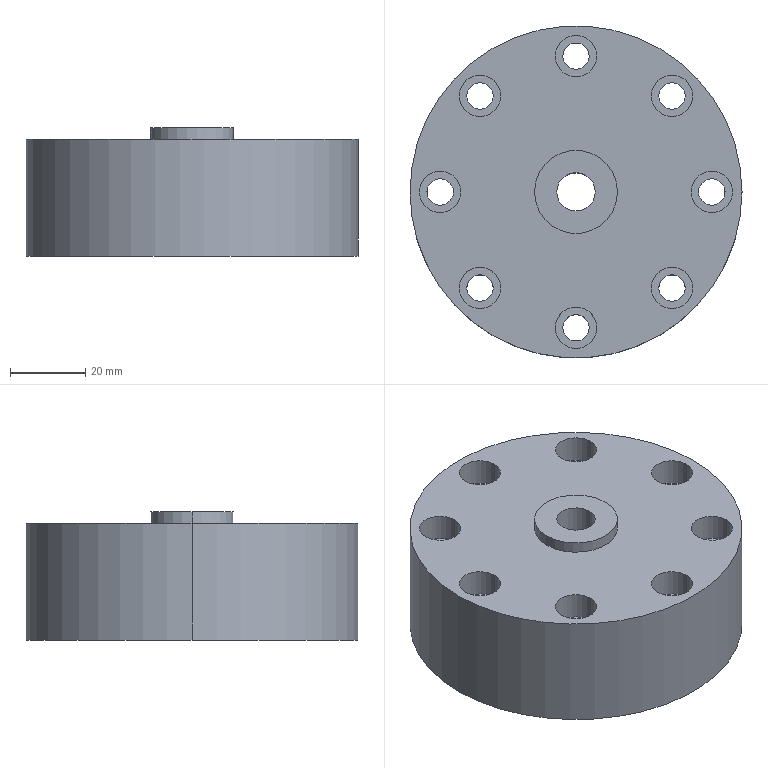Part | SolidWorks | features BaseBody 1 | 1 solid | 49 faces | box 88 x 88 x 34 mm | volume 174107 mm3 | cylinder 38 | plane 11 | commonest cylinder face diameters 7 x16 11 x16 10.2 x2 22 x2 88 x2
STEP:
#1=CARTESIAN_POINT('',(-44.,-15.,364.481));
#2=VERTEX_POINT('',#1);
#3=CARTESIAN_POINT('',(44.,-15.,364.481));
#4=VERTEX_POINT('',#3);
#5=CARTESIAN_POINT('',(0.,-15.,364.481));
#6=DIRECTION('',(0.,0.,-1.));
#7=DIRECTION('',(-1.,0.,0.));
#8=AXIS2_PLACEMENT_3D('',#5,#6,#7);
#9=CIRCLE('',#8,44.);
#10=EDGE_CURVE('',#2,#4,#9,.T.);
#11=ORIENTED_EDGE('',*,*,#10,.T.);
#12=CARTESIAN_POINT('',(44.,-15.,333.481));
#13=VERTEX_POINT('',#12);
#14=CARTESIAN_POINT('',(44.,-15.,364.481));
#15=DIRECTION('',(0.,0.,-1.));
#16=VECTOR('',#15,1000.);
#17=LINE('',#14,#16);
#18=EDGE_CURVE('',#4,#13,#17,.T.);
#19=ORIENTED_EDGE('',*,*,#18,.T.);
#20=CARTESIAN_POINT('',(-44.,-15.,333.481));
#21=VERTEX_POINT('',#20);
#22=CARTESIAN_POINT('',(0.,-15.,333.481));
#23=DIRECTION('',(0.,0.,1.));
#24=DIRECTION('',(-1.,0.,0.));
#25=AXIS2_PLACEMENT_3D('',#22,#23,#24);
#26=CIRCLE('',#25,44.);
#27=EDGE_CURVE('',#13,#21,#26,.T.);
#28=ORIENTED_EDGE('',*,*,#27,.T.);
#29=CARTESIAN_POINT('',(-44.,-15.,364.481));
#30=DIRECTION('',(0.,0.,-1.));
#31=VECTOR('',#30,1000.);
#32=LINE('',#29,#31);
#33=EDGE_CURVE('',#2,#21,#32,.T.);
#34=ORIENTED_EDGE('',*,*,#33,.F.);
#35=EDGE_LOOP('',(#11,#19,#28,#34));
#36=FACE_OUTER_BOUND('',#35,.T.);
#37=CARTESIAN_POINT('',(0.,-15.,364.481));
#38=DIRECTION('',(0.,0.,-1.));
#39=DIRECTION('',(-1.,0.,0.));
#40=AXIS2_PLACEMENT_3D('',#37,#38,#39);
#41=CYLINDRICAL_SURFACE('',#40,44.);
#42=ADVANCED_FACE('',(#36),#41,.T.);
#43=CARTESIAN_POINT('',(5.1,-15.,333.481));
#44=VERTEX_POINT('',#43);
#45=CARTESIAN_POINT('',(-5.1,-15.,333.481));
#46=VERTEX_POINT('',#45);
#47=CARTESIAN_POINT('',(0.,-15.,333.481));
#48=DIRECTION('',(0.,0.,-1.));
#49=DIRECTION('',(1.,0.,0.));
#50=AXIS2_PLACEMENT_3D('',#47,#48,#49);
#51=CIRCLE('',#50,5.1);
#52=EDGE_CURVE('',#44,#46,#51,.T.);
#53=ORIENTED_EDGE('',*,*,#52,.T.);
#54=CARTESIAN_POINT('',(-5.1,-15.,367.481));
#55=VERTEX_POINT('',#54);
#56=CARTESIAN_POINT('',(-5.1,-15.,367.481));
#57=DIRECTION('',(0.,0.,1.));
#58=VECTOR('',#57,1000.);
#59=LINE('',#56,#58);
#60=EDGE_CURVE('',#46,#55,#59,.T.);
#61=ORIENTED_EDGE('',*,*,#60,.T.);
#62=CARTESIAN_POINT('',(5.1,-15.,367.481));
#63=VERTEX_POINT('',#62);
#64=CARTESIAN_POINT('',(0.,-15.,367.481));
#65=DIRECTION('',(0.,0.,-1.));
#66=DIRECTION('',(1.,0.,0.));
#67=AXIS2_PLACEMENT_3D('',#64,#65,#66);
#68=CIRCLE('',#67,5.1);
#69=EDGE_CURVE('',#63,#55,#68,.T.);
#70=ORIENTED_EDGE('',*,*,#69,.F.);
#71=CARTESIAN_POINT('',(5.1,-15.,367.481));
#72=DIRECTION('',(0.,0.,1.));
#73=VECTOR('',#72,1000.);
#74=LINE('',#71,#73);
#75=EDGE_CURVE('',#44,#63,#74,.T.);
#76=ORIENTED_EDGE('',*,*,#75,.F.);
#77=EDGE_LOOP('',(#53,#61,#70,#76));
#78=FACE_OUTER_BOUND('',#77,.T.);
#79=CARTESIAN_POINT('',(0.,-15.,367.481));
#80=DIRECTION('',(0.,0.,1.));
#81=DIRECTION('',(1.,0.,0.));
#82=AXIS2_PLACEMENT_3D('',#79,#80,#81);
#83=CYLINDRICAL_SURFACE('',#82,5.1);
#84=ADVANCED_FACE('',(#78),#83,.F.);
#85=CARTESIAN_POINT('',(39.5,-15.,333.481));
#86=VERTEX_POINT('',#85);
#87=CARTESIAN_POINT('',(32.5,-15.,333.481));
#88=VERTEX_POINT('',#87);
#89=CARTESIAN_POINT('',(36.,-15.,333.481));
#90=DIRECTION('',(0.,0.,-1.));
#91=DIRECTION('',(1.,0.,0.));
#92=AXIS2_PLACEMENT_3D('',#89,#90,#91);
#93=CIRCLE('',#92,3.5);
#94=EDGE_CURVE('',#86,#88,#93,.T.);
#95=ORIENTED_EDGE('',*,*,#94,.T.);
#96=CARTESIAN_POINT('',(32.5,-15.,357.281));
#97=VERTEX_POINT('',#96);
#98=CARTESIAN_POINT('',(32.5,-15.,333.481));
#99=DIRECTION('',(0.,0.,1.));
#100=VECTOR('',#99,1000.);
#101=LINE('',#98,#100);
#102=EDGE_CURVE('',#88,#97,#101,.T.);
#103=ORIENTED_EDGE('',*,*,#102,.T.);
#104=CARTESIAN_POINT('',(39.5,-15.,357.281));
#105=VERTEX_POINT('',#104);
#106=CARTESIAN_POINT('',(36.,-15.,357.281));
#107=DIRECTION('',(0.,0.,-1.));
#108=DIRECTION('',(1.,0.,0.));
#109=AXIS2_PLACEMENT_3D('',#106,#107,#108);
#110=CIRCLE('',#109,3.5);
#111=EDGE_CURVE('',#105,#97,#110,.T.);
#112=ORIENTED_EDGE('',*,*,#111,.F.);
#113=CARTESIAN_POINT('',(39.5,-15.,333.481));
#114=DIRECTION('',(0.,0.,1.));
#115=VECTOR('',#114,1000.);
#116=LINE('',#113,#115);
#117=EDGE_CURVE('',#86,#105,#116,.T.);
#118=ORIENTED_EDGE('',*,*,#117,.F.);
#119=EDGE_LOOP('',(#95,#103,#112,#118));
#120=FACE_OUTER_BOUND('',#119,.T.);
#121=CARTESIAN_POINT('',(36.,-15.,333.481));
#122=DIRECTION('',(0.,0.,1.));
#123=DIRECTION('',(1.,0.,0.));
#124=AXIS2_PLACEMENT_3D('',#121,#122,#123);
#125=CYLINDRICAL_SURFACE('',#124,3.5);
#126=ADVANCED_FACE('',(#120),#125,.F.);
#127=CARTESIAN_POINT('',(28.956,10.456,333.481));
#128=VERTEX_POINT('',#127);
#129=CARTESIAN_POINT('',(21.956,10.456,333.481));
#130=VERTEX_POINT('',#129);
#131=CARTESIAN_POINT('',(25.456,10.456,333.481));
#132=DIRECTION('',(0.,0.,-1.));
#133=DIRECTION('',(1.,0.,0.));
#134=AXIS2_PLACEMENT_3D('',#131,#132,#133);
#135=CIRCLE('',#134,3.5);
#136=EDGE_CURVE('',#128,#130,#135,.T.);
#137=ORIENTED_EDGE('',*,*,#136,.T.);
#138=CARTESIAN_POINT('',(21.956,10.456,357.281));
#139=VERTEX_POINT('',#138);
#140=CARTESIAN_POINT('',(21.956,10.456,333.481));
#141=DIRECTION('',(0.,0.,1.));
#142=VECTOR('',#141,1000.);
#143=LINE('',#140,#142);
#144=EDGE_CURVE('',#130,#139,#143,.T.);
#145=ORIENTED_EDGE('',*,*,#144,.T.);
#146=CARTESIAN_POINT('',(28.956,10.456,357.281));
#147=VERTEX_POINT('',#146);
#148=CARTESIAN_POINT('',(25.456,10.456,357.281));
#149=DIRECTION('',(0.,0.,-1.));
#150=DIRECTION('',(1.,0.,0.));
#151=AXIS2_PLACEMENT_3D('',#148,#149,#150);
#152=CIRCLE('',#151,3.5);
#153=EDGE_CURVE('',#147,#139,#152,.T.);
#154=ORIENTED_EDGE('',*,*,#153,.F.);
#155=CARTESIAN_POINT('',(28.956,10.456,333.481));
#156=DIRECTION('',(0.,0.,1.));
#157=VECTOR('',#156,1000.);
#158=LINE('',#155,#157);
#159=EDGE_CURVE('',#128,#147,#158,.T.);
#160=ORIENTED_EDGE('',*,*,#159,.F.);
#161=EDGE_LOOP('',(#137,#145,#154,#160));
#162=FACE_OUTER_BOUND('',#161,.T.);
#163=CARTESIAN_POINT('',(25.456,10.456,333.481));
#164=DIRECTION('',(0.,0.,1.));
#165=DIRECTION('',(1.,0.,0.));
#166=AXIS2_PLACEMENT_3D('',#163,#164,#165);
#167=CYLINDRICAL_SURFACE('',#166,3.5);
#168=ADVANCED_FACE('',(#162),#167,.F.);
#169=CARTESIAN_POINT('',(3.5,21.,333.481));
#170=VERTEX_POINT('',#169);
#171=CARTESIAN_POINT('',(-3.5,21.,333.481));
#172=VERTEX_POINT('',#171);
#173=CARTESIAN_POINT('',(0.,21.,333.481));
#174=DIRECTION('',(0.,0.,-1.));
#175=DIRECTION('',(1.,0.,0.));
#176=AXIS2_PLACEMENT_3D('',#173,#174,#175);
#177=CIRCLE('',#176,3.5);
#178=EDGE_CURVE('',#170,#172,#177,.T.);
#179=ORIENTED_EDGE('',*,*,#178,.T.);
#180=CARTESIAN_POINT('',(-3.5,21.,357.281));
#181=VERTEX_POINT('',#180);
#182=CARTESIAN_POINT('',(-3.5,21.,333.481));
#183=DIRECTION('',(0.,0.,1.));
#184=VECTOR('',#183,1000.);
#185=LINE('',#182,#184);
#186=EDGE_CURVE('',#172,#181,#185,.T.);
#187=ORIENTED_EDGE('',*,*,#186,.T.);
#188=CARTESIAN_POINT('',(3.5,21.,357.281));
#189=VERTEX_POINT('',#188);
#190=CARTESIAN_POINT('',(0.,21.,357.281));
#191=DIRECTION('',(0.,0.,-1.));
#192=DIRECTION('',(1.,0.,0.));
#193=AXIS2_PLACEMENT_3D('',#190,#191,#192);
#194=CIRCLE('',#193,3.5);
#195=EDGE_CURVE('',#189,#181,#194,.T.);
#196=ORIENTED_EDGE('',*,*,#195,.F.);
#197=CARTESIAN_POINT('',(3.5,21.,333.481));
#198=DIRECTION('',(0.,0.,1.));
#199=VECTOR('',#198,1000.);
#200=LINE('',#197,#199);
#201=EDGE_CURVE('',#170,#189,#200,.T.);
#202=ORIENTED_EDGE('',*,*,#201,.F.);
#203=EDGE_LOOP('',(#179,#187,#196,#202));
#204=FACE_OUTER_BOUND('',#203,.T.);
#205=CARTESIAN_POINT('',(0.,21.,333.481));
#206=DIRECTION('',(0.,0.,1.));
#207=DIRECTION('',(1.,0.,0.));
#208=AXIS2_PLACEMENT_3D('',#205,#206,#207);
#209=CYLINDRICAL_SURFACE('',#208,3.5);
#210=ADVANCED_FACE('',(#204),#209,.F.);
#211=CARTESIAN_POINT('',(-21.956,10.456,333.481));
#212=VERTEX_POINT('',#211);
#213=CARTESIAN_POINT('',(-28.956,10.456,333.481));
#214=VERTEX_POINT('',#213);
#215=CARTESIAN_POINT('',(-25.456,10.456,333.481));
#216=DIRECTION('',(0.,0.,-1.));
#217=DIRECTION('',(1.,0.,0.));
#218=AXIS2_PLACEMENT_3D('',#215,#216,#217);
#219=CIRCLE('',#218,3.5);
#220=EDGE_CURVE('',#212,#214,#219,.T.);
#221=ORIENTED_EDGE('',*,*,#220,.T.);
#222=CARTESIAN_POINT('',(-28.956,10.456,357.281));
#223=VERTEX_POINT('',#222);
#224=CARTESIAN_POINT('',(-28.956,10.456,333.481));
#225=DIRECTION('',(0.,0.,1.));
#226=VECTOR('',#225,1000.);
#227=LINE('',#224,#226);
#228=EDGE_CURVE('',#214,#223,#227,.T.);
#229=ORIENTED_EDGE('',*,*,#228,.T.);
#230=CARTESIAN_POINT('',(-21.956,10.456,357.281));
#231=VERTEX_POINT('',#230);
#232=CARTESIAN_POINT('',(-25.456,10.456,357.281));
#233=DIRECTION('',(0.,0.,-1.));
#234=DIRECTION('',(1.,0.,0.));
#235=AXIS2_PLACEMENT_3D('',#232,#233,#234);
#236=CIRCLE('',#235,3.5);
#237=EDGE_CURVE('',#231,#223,#236,.T.);
#238=ORIENTED_EDGE('',*,*,#237,.F.);
#239=CARTESIAN_POINT('',(-21.956,10.456,333.481));
#240=DIRECTION('',(0.,0.,1.));
#241=VECTOR('',#240,1000.);
#242=LINE('',#239,#241);
#243=EDGE_CURVE('',#212,#231,#242,.T.);
#244=ORIENTED_EDGE('',*,*,#243,.F.);
#245=EDGE_LOOP('',(#221,#229,#238,#244));
#246=FACE_OUTER_BOUND('',#245,.T.);
#247=CARTESIAN_POINT('',(-25.456,10.456,333.481));
#248=DIRECTION('',(0.,0.,1.));
#249=DIRECTION('',(1.,0.,0.));
#250=AXIS2_PLACEMENT_3D('',#247,#248,#249);
#251=CYLINDRICAL_SURFACE('',#250,3.5);
#252=ADVANCED_FACE('',(#246),#251,.F.);
#253=CARTESIAN_POINT('',(-32.5,-15.,333.481));
#254=VERTEX_POINT('',#253);
#255=CARTESIAN_POINT('',(-39.5,-15.,333.481));
#256=VERTEX_POINT('',#255);
#257=CARTESIAN_POINT('',(-36.,-15.,333.481));
#258=DIRECTION('',(0.,0.,-1.));
#259=DIRECTION('',(1.,0.,0.));
#260=AXIS2_PLACEMENT_3D('',#257,#258,#259);
#261=CIRCLE('',#260,3.5);
#262=EDGE_CURVE('',#254,#256,#261,.T.);
#263=ORIENTED_EDGE('',*,*,#262,.T.);
#264=CARTESIAN_POINT('',(-39.5,-15.,357.281));
#265=VERTEX_POINT('',#264);
#266=CARTESIAN_POINT('',(-39.5,-15.,333.481));
#267=DIRECTION('',(0.,0.,1.));
#268=VECTOR('',#267,1000.);
#269=LINE('',#266,#268);
#270=EDGE_CURVE('',#256,#265,#269,.T.);
#271=ORIENTED_EDGE('',*,*,#270,.T.);
#272=CARTESIAN_POINT('',(-32.5,-15.,357.281));
#273=VERTEX_POINT('',#272);
#274=CARTESIAN_POINT('',(-36.,-15.,357.281));
#275=DIRECTION('',(0.,0.,-1.));
#276=DIRECTION('',(1.,0.,0.));
#277=AXIS2_PLACEMENT_3D('',#274,#275,#276);
#278=CIRCLE('',#277,3.5);
#279=EDGE_CURVE('',#273,#265,#278,.T.);
#280=ORIENTED_EDGE('',*,*,#279,.F.);
#281=CARTESIAN_POINT('',(-32.5,-15.,333.481));
#282=DIRECTION('',(0.,0.,1.));
#283=VECTOR('',#282,1000.);
#284=LINE('',#281,#283);
#285=EDGE_CURVE('',#254,#273,#284,.T.);
#286=ORIENTED_EDGE('',*,*,#285,.F.);
#287=EDGE_LOOP('',(#263,#271,#280,#286));
#288=FACE_OUTER_BOUND('',#287,.T.);
#289=CARTESIAN_POINT('',(-36.,-15.,333.481));
#290=DIRECTION('',(0.,0.,1.));
#291=DIRECTION('',(1.,0.,0.));
#292=AXIS2_PLACEMENT_3D('',#289,#290,#291);
#293=CYLINDRICAL_SURFACE('',#292,3.5);
#294=ADVANCED_FACE('',(#288),#293,.F.);
#295=CARTESIAN_POINT('',(-21.956,-40.456,333.481));
#296=VERTEX_POINT('',#295);
#297=CARTESIAN_POINT('',(-28.956,-40.456,333.481));
#298=VERTEX_POINT('',#297);
#299=CARTESIAN_POINT('',(-25.456,-40.456,333.481));
#300=DIRECTION('',(0.,0.,-1.));
#301=DIRECTION('',(1.,0.,0.));
#302=AXIS2_PLACEMENT_3D('',#299,#300,#301);
#303=CIRCLE('',#302,3.5);
#304=EDGE_CURVE('',#296,#298,#303,.T.);
#305=ORIENTED_EDGE('',*,*,#304,.T.);
#306=CARTESIAN_POINT('',(-28.956,-40.456,357.281));
#307=VERTEX_POINT('',#306);
#308=CARTESIAN_POINT('',(-28.956,-40.456,333.481));
#309=DIRECTION('',(0.,0.,1.));
#310=VECTOR('',#309,1000.);
#311=LINE('',#308,#310);
#312=EDGE_CURVE('',#298,#307,#311,.T.);
#313=ORIENTED_EDGE('',*,*,#312,.T.);
#314=CARTESIAN_POINT('',(-21.956,-40.456,357.281));
#315=VERTEX_POINT('',#314);
#316=CARTESIAN_POINT('',(-25.456,-40.456,357.281));
#317=DIRECTION('',(0.,0.,-1.));
#318=DIRECTION('',(1.,0.,0.));
#319=AXIS2_PLACEMENT_3D('',#316,#317,#318);
#320=CIRCLE('',#319,3.5);
#321=EDGE_CURVE('',#315,#307,#320,.T.);
#322=ORIENTED_EDGE('',*,*,#321,.F.);
#323=CARTESIAN_POINT('',(-21.956,-40.456,333.481));
#324=DIRECTION('',(0.,0.,1.));
#325=VECTOR('',#324,1000.);
#326=LINE('',#323,#325);
#327=EDGE_CURVE('',#296,#315,#326,.T.);
#328=ORIENTED_EDGE('',*,*,#327,.F.);
#329=EDGE_LOOP('',(#305,#313,#322,#328));
#330=FACE_OUTER_BOUND('',#329,.T.);
#331=CARTESIAN_POINT('',(-25.456,-40.456,333.481));
#332=DIRECTION('',(0.,0.,1.));
#333=DIRECTION('',(1.,0.,0.));
#334=AXIS2_PLACEMENT_3D('',#331,#332,#333);
#335=CYLINDRICAL_SURFACE('',#334,3.5);
#336=ADVANCED_FACE('',(#330),#335,.F.);
#337=CARTESIAN_POINT('',(3.5,-51.,333.481));
#338=VERTEX_POINT('',#337);
#339=CARTESIAN_POINT('',(-3.5,-51.,333.481));
#340=VERTEX_POINT('',#339);
#341=CARTESIAN_POINT('',(0.,-51.,333.481));
#342=DIRECTION('',(0.,0.,-1.));
#343=DIRECTION('',(1.,0.,0.));
#344=AXIS2_PLACEMENT_3D('',#341,#342,#343);
#345=CIRCLE('',#344,3.5);
#346=EDGE_CURVE('',#338,#340,#345,.T.);
#347=ORIENTED_EDGE('',*,*,#346,.T.);
#348=CARTESIAN_POINT('',(-3.5,-51.,357.281));
#349=VERTEX_POINT('',#348);
#350=CARTESIAN_POINT('',(-3.5,-51.,333.481));
#351=DIRECTION('',(0.,0.,1.));
#352=VECTOR('',#351,1000.);
#353=LINE('',#350,#352);
#354=EDGE_CURVE('',#340,#349,#353,.T.);
#355=ORIENTED_EDGE('',*,*,#354,.T.);
#356=CARTESIAN_POINT('',(3.5,-51.,357.281));
#357=VERTEX_POINT('',#356);
#358=CARTESIAN_POINT('',(0.,-51.,357.281));
#359=DIRECTION('',(0.,0.,-1.));
#360=DIRECTION('',(1.,0.,0.));
#361=AXIS2_PLACEMENT_3D('',#358,#359,#360);
#362=CIRCLE('',#361,3.5);
#363=EDGE_CURVE('',#357,#349,#362,.T.);
#364=ORIENTED_EDGE('',*,*,#363,.F.);
#365=CARTESIAN_POINT('',(3.5,-51.,333.481));
#366=DIRECTION('',(0.,0.,1.));
#367=VECTOR('',#366,1000.);
#368=LINE('',#365,#367);
#369=EDGE_CURVE('',#338,#357,#368,.T.);
#370=ORIENTED_EDGE('',*,*,#369,.F.);
#371=EDGE_LOOP('',(#347,#355,#364,#370));
#372=FACE_OUTER_BOUND('',#371,.T.);
#373=CARTESIAN_POINT('',(0.,-51.,333.481));
#374=DIRECTION('',(0.,0.,1.));
#375=DIRECTION('',(1.,0.,0.));
#376=AXIS2_PLACEMENT_3D('',#373,#374,#375);
#377=CYLINDRICAL_SURFACE('',#376,3.5);
#378=ADVANCED_FACE('',(#372),#377,.F.);
#379=CARTESIAN_POINT('',(28.956,-40.456,333.481));
#380=VERTEX_POINT('',#379);
#381=CARTESIAN_POINT('',(21.956,-40.456,333.481));
#382=VERTEX_POINT('',#381);
#383=CARTESIAN_POINT('',(25.456,-40.456,333.481));
#384=DIRECTION('',(0.,0.,-1.));
#385=DIRECTION('',(1.,0.,0.));
#386=AXIS2_PLACEMENT_3D('',#383,#384,#385);
#387=CIRCLE('',#386,3.5);
#388=EDGE_CURVE('',#380,#382,#387,.T.);
#389=ORIENTED_EDGE('',*,*,#388,.T.);
#390=CARTESIAN_POINT('',(21.956,-40.456,357.281));
#391=VERTEX_POINT('',#390);
#392=CARTESIAN_POINT('',(21.956,-40.456,333.481));
#393=DIRECTION('',(0.,0.,1.));
#394=VECTOR('',#393,1000.);
#395=LINE('',#392,#394);
#396=EDGE_CURVE('',#382,#391,#395,.T.);
#397=ORIENTED_EDGE('',*,*,#396,.T.);
#398=CARTESIAN_POINT('',(28.956,-40.456,357.281));
#399=VERTEX_POINT('',#398);
#400=CARTESIAN_POINT('',(25.456,-40.456,357.281));
#401=DIRECTION('',(0.,0.,-1.));
#402=DIRECTION('',(1.,0.,0.));
#403=AXIS2_PLACEMENT_3D('',#400,#401,#402);
#404=CIRCLE('',#403,3.5);
#405=EDGE_CURVE('',#399,#391,#404,.T.);
#406=ORIENTED_EDGE('',*,*,#405,.F.);
#407=CARTESIAN_POINT('',(28.956,-40.456,333.481));
#408=DIRECTION('',(0.,0.,1.));
#409=VECTOR('',#408,1000.);
#410=LINE('',#407,#409);
#411=EDGE_CURVE('',#380,#399,#410,.T.);
#412=ORIENTED_EDGE('',*,*,#411,.F.);
#413=EDGE_LOOP('',(#389,#397,#406,#412));
#414=FACE_OUTER_BOUND('',#413,.T.);
#415=CARTESIAN_POINT('',(25.456,-40.456,333.481));
#416=DIRECTION('',(0.,0.,1.));
#417=DIRECTION('',(1.,0.,0.));
#418=AXIS2_PLACEMENT_3D('',#415,#416,#417);
#419=CYLINDRICAL_SURFACE('',#418,3.5);
#420=ADVANCED_FACE('',(#414),#419,.F.);
#421=CARTESIAN_POINT('',(11.,-15.,367.481));
#422=VERTEX_POINT('',#421);
#423=CARTESIAN_POINT('',(-11.,-15.,367.481));
#424=VERTEX_POINT('',#423);
#425=CARTESIAN_POINT('',(0.,-15.,367.481));
#426=DIRECTION('',(0.,0.,1.));
#427=DIRECTION('',(-1.,0.,0.));
#428=AXIS2_PLACEMENT_3D('',#425,#426,#427);
#429=CIRCLE('',#428,11.);
#430=EDGE_CURVE('',#422,#424,#429,.T.);
#431=ORIENTED_EDGE('',*,*,#430,.F.);
#432=CARTESIAN_POINT('',(11.,-15.,364.481));
#433=VERTEX_POINT('',#432);
#434=CARTESIAN_POINT('',(11.,-15.,367.481));
#435=DIRECTION('',(0.,0.,-1.));
#436=VECTOR('',#435,1000.);
#437=LINE('',#434,#436);
#438=EDGE_CURVE('',#422,#433,#437,.T.);
#439=ORIENTED_EDGE('',*,*,#438,.T.);
#440=CARTESIAN_POINT('',(-11.,-15.,364.481));
#441=VERTEX_POINT('',#440);
#442=CARTESIAN_POINT('',(0.,-15.,364.481));
#443=DIRECTION('',(0.,0.,-1.));
#444=DIRECTION('',(-1.,0.,0.));
#445=AXIS2_PLACEMENT_3D('',#442,#443,#444);
#446=CIRCLE('',#445,11.);
#447=EDGE_CURVE('',#441,#433,#446,.T.);
#448=ORIENTED_EDGE('',*,*,#447,.F.);
#449=CARTESIAN_POINT('',(-11.,-15.,367.481));
#450=DIRECTION('',(0.,0.,-1.));
#451=VECTOR('',#450,1000.);
#452=LINE('',#449,#451);
#453=EDGE_CURVE('',#424,#441,#452,.T.);
#454=ORIENTED_EDGE('',*,*,#453,.F.);
#455=EDGE_LOOP('',(#431,#439,#448,#454));
#456=FACE_OUTER_BOUND('',#455,.T.);
#457=CARTESIAN_POINT('',(0.,-15.,367.481));
#458=DIRECTION('',(0.,0.,-1.));
#459=DIRECTION('',(-1.,0.,0.));
#460=AXIS2_PLACEMENT_3D('',#457,#458,#459);
#461=CYLINDRICAL_SURFACE('',#460,11.);
#462=ADVANCED_FACE('',(#456),#461,.T.);
#463=CARTESIAN_POINT('',(30.5,-15.,357.281));
#464=VERTEX_POINT('',#463);
#465=CARTESIAN_POINT('',(41.5,-15.,357.281));
#466=VERTEX_POINT('',#465);
#467=CARTESIAN_POINT('',(36.,-15.,357.281));
#468=DIRECTION('',(0.,0.,1.));
#469=DIRECTION('',(1.,0.,0.));
#470=AXIS2_PLACEMENT_3D('',#467,#468,#469);
#471=CIRCLE('',#470,5.5);
#472=EDGE_CURVE('',#464,#466,#471,.T.);
#473=ORIENTED_EDGE('',*,*,#472,.F.);
#474=CARTESIAN_POINT('',(30.5,-15.,364.481));
#475=VERTEX_POINT('',#474);
#476=CARTESIAN_POINT('',(30.5,-15.,357.281));
#477=DIRECTION('',(0.,0.,1.));
#478=VECTOR('',#477,1000.);
#479=LINE('',#476,#478);
#480=EDGE_CURVE('',#464,#475,#479,.T.);
#481=ORIENTED_EDGE('',*,*,#480,.T.);
#482=CARTESIAN_POINT('',(41.5,-15.,364.481));
#483=VERTEX_POINT('',#482);
#484=CARTESIAN_POINT('',(36.,-15.,364.481));
#485=DIRECTION('',(0.,0.,-1.));
#486=DIRECTION('',(1.,0.,0.));
#487=AXIS2_PLACEMENT_3D('',#484,#485,#486);
#488=CIRCLE('',#487,5.5);
#489=EDGE_CURVE('',#483,#475,#488,.T.);
#490=ORIENTED_EDGE('',*,*,#489,.F.);
#491=CARTESIAN_POINT('',(41.5,-15.,357.281));
#492=DIRECTION('',(0.,0.,1.));
#493=VECTOR('',#492,1000.);
#494=LINE('',#491,#493);
#495=EDGE_CURVE('',#466,#483,#494,.T.);
#496=ORIENTED_EDGE('',*,*,#495,.F.);
#497=EDGE_LOOP('',(#473,#481,#490,#496));
#498=FACE_OUTER_BOUND('',#497,.T.);
#499=CARTESIAN_POINT('',(36.,-15.,357.281));
#500=DIRECTION('',(0.,0.,1.));
#501=DIRECTION('',(1.,0.,0.));
#502=AXIS2_PLACEMENT_3D('',#499,#500,#501);
#503=CYLINDRICAL_SURFACE('',#502,5.5);
#504=ADVANCED_FACE('',(#498),#503,.F.);
#505=CARTESIAN_POINT('',(19.956,10.456,357.281));
#506=VERTEX_POINT('',#505);
#507=CARTESIAN_POINT('',(30.956,10.456,357.281));
#508=VERTEX_POINT('',#507);
#509=CARTESIAN_POINT('',(25.456,10.456,357.281));
#510=DIRECTION('',(0.,0.,1.));
#511=DIRECTION('',(1.,0.,0.));
#512=AXIS2_PLACEMENT_3D('',#509,#510,#511);
#513=CIRCLE('',#512,5.5);
#514=EDGE_CURVE('',#506,#508,#513,.T.);
#515=ORIENTED_EDGE('',*,*,#514,.F.);
#516=CARTESIAN_POINT('',(19.956,10.456,364.481));
#517=VERTEX_POINT('',#516);
#518=CARTESIAN_POINT('',(19.956,10.456,357.281));
#519=DIRECTION('',(0.,0.,1.));
#520=VECTOR('',#519,1000.);
#521=LINE('',#518,#520);
#522=EDGE_CURVE('',#506,#517,#521,.T.);
#523=ORIENTED_EDGE('',*,*,#522,.T.);
#524=CARTESIAN_POINT('',(30.956,10.456,364.481));
#525=VERTEX_POINT('',#524);
#526=CARTESIAN_POINT('',(25.456,10.456,364.481));
#527=DIRECTION('',(0.,0.,-1.));
#528=DIRECTION('',(1.,0.,0.));
#529=AXIS2_PLACEMENT_3D('',#526,#527,#528);
#530=CIRCLE('',#529,5.5);
#531=EDGE_CURVE('',#525,#517,#530,.T.);
#532=ORIENTED_EDGE('',*,*,#531,.F.);
#533=CARTESIAN_POINT('',(30.956,10.456,357.281));
#534=DIRECTION('',(0.,0.,1.));
#535=VECTOR('',#534,1000.);
#536=LINE('',#533,#535);
#537=EDGE_CURVE('',#508,#525,#536,.T.);
#538=ORIENTED_EDGE('',*,*,#537,.F.);
#539=EDGE_LOOP('',(#515,#523,#532,#538));
#540=FACE_OUTER_BOUND('',#539,.T.);
#541=CARTESIAN_POINT('',(25.456,10.456,357.281));
#542=DIRECTION('',(0.,0.,1.));
#543=DIRECTION('',(1.,0.,0.));
#544=AXIS2_PLACEMENT_3D('',#541,#542,#543);
#545=CYLINDRICAL_SURFACE('',#544,5.5);
#546=ADVANCED_FACE('',(#540),#545,.F.);
#547=CARTESIAN_POINT('',(-5.5,21.,357.281));
#548=VERTEX_POINT('',#547);
#549=CARTESIAN_POINT('',(5.5,21.,357.281));
#550=VERTEX_POINT('',#549);
#551=CARTESIAN_POINT('',(0.,21.,357.281));
#552=DIRECTION('',(0.,0.,1.));
#553=DIRECTION('',(1.,0.,0.));
#554=AXIS2_PLACEMENT_3D('',#551,#552,#553);
#555=CIRCLE('',#554,5.5);
#556=EDGE_CURVE('',#548,#550,#555,.T.);
#557=ORIENTED_EDGE('',*,*,#556,.F.);
#558=CARTESIAN_POINT('',(-5.5,21.,364.481));
#559=VERTEX_POINT('',#558);
#560=CARTESIAN_POINT('',(-5.5,21.,357.281));
#561=DIRECTION('',(0.,0.,1.));
#562=VECTOR('',#561,1000.);
#563=LINE('',#560,#562);
#564=EDGE_CURVE('',#548,#559,#563,.T.);
#565=ORIENTED_EDGE('',*,*,#564,.T.);
#566=CARTESIAN_POINT('',(5.5,21.,364.481));
#567=VERTEX_POINT('',#566);
#568=CARTESIAN_POINT('',(0.,21.,364.481));
#569=DIRECTION('',(0.,0.,-1.));
#570=DIRECTION('',(1.,0.,0.));
#571=AXIS2_PLACEMENT_3D('',#568,#569,#570);
#572=CIRCLE('',#571,5.5);
#573=EDGE_CURVE('',#567,#559,#572,.T.);
#574=ORIENTED_EDGE('',*,*,#573,.F.);
#575=CARTESIAN_POINT('',(5.5,21.,357.281));
#576=DIRECTION('',(0.,0.,1.));
#577=VECTOR('',#576,1000.);
#578=LINE('',#575,#577);
#579=EDGE_CURVE('',#550,#567,#578,.T.);
#580=ORIENTED_EDGE('',*,*,#579,.F.);
#581=EDGE_LOOP('',(#557,#565,#574,#580));
#582=FACE_OUTER_BOUND('',#581,.T.);
#583=CARTESIAN_POINT('',(0.,21.,357.281));
#584=DIRECTION('',(0.,0.,1.));
#585=DIRECTION('',(1.,0.,0.));
#586=AXIS2_PLACEMENT_3D('',#583,#584,#585);
#587=CYLINDRICAL_SURFACE('',#586,5.5);
#588=ADVANCED_FACE('',(#582),#587,.F.);
#589=CARTESIAN_POINT('',(-30.956,10.456,357.281));
#590=VERTEX_POINT('',#589);
#591=CARTESIAN_POINT('',(-19.956,10.456,357.281));
#592=VERTEX_POINT('',#591);
#593=CARTESIAN_POINT('',(-25.456,10.456,357.281));
#594=DIRECTION('',(0.,0.,1.));
#595=DIRECTION('',(1.,0.,0.));
#596=AXIS2_PLACEMENT_3D('',#593,#594,#595);
#597=CIRCLE('',#596,5.5);
#598=EDGE_CURVE('',#590,#592,#597,.T.);
#599=ORIENTED_EDGE('',*,*,#598,.F.);
#600=CARTESIAN_POINT('',(-30.956,10.456,364.481));
#601=VERTEX_POINT('',#600);
#602=CARTESIAN_POINT('',(-30.956,10.456,357.281));
#603=DIRECTION('',(0.,0.,1.));
#604=VECTOR('',#603,1000.);
#605=LINE('',#602,#604);
#606=EDGE_CURVE('',#590,#601,#605,.T.);
#607=ORIENTED_EDGE('',*,*,#606,.T.);
#608=CARTESIAN_POINT('',(-19.956,10.456,364.481));
#609=VERTEX_POINT('',#608);
#610=CARTESIAN_POINT('',(-25.456,10.456,364.481));
#611=DIRECTION('',(0.,0.,-1.));
#612=DIRECTION('',(1.,0.,0.));
#613=AXIS2_PLACEMENT_3D('',#610,#611,#612);
#614=CIRCLE('',#613,5.5);
#615=EDGE_CURVE('',#609,#601,#614,.T.);
#616=ORIENTED_EDGE('',*,*,#615,.F.);
#617=CARTESIAN_POINT('',(-19.956,10.456,357.281));
#618=DIRECTION('',(0.,0.,1.));
#619=VECTOR('',#618,1000.);
#620=LINE('',#617,#619);
#621=EDGE_CURVE('',#592,#609,#620,.T.);
#622=ORIENTED_EDGE('',*,*,#621,.F.);
#623=EDGE_LOOP('',(#599,#607,#616,#622));
#624=FACE_OUTER_BOUND('',#623,.T.);
#625=CARTESIAN_POINT('',(-25.456,10.456,357.281));
#626=DIRECTION('',(0.,0.,1.));
#627=DIRECTION('',(1.,0.,0.));
#628=AXIS2_PLACEMENT_3D('',#625,#626,#627);
#629=CYLINDRICAL_SURFACE('',#628,5.5);
#630=ADVANCED_FACE('',(#624),#629,.F.);
#631=CARTESIAN_POINT('',(-41.5,-15.,357.281));
#632=VERTEX_POINT('',#631);
#633=CARTESIAN_POINT('',(-30.5,-15.,357.281));
#634=VERTEX_POINT('',#633);
#635=CARTESIAN_POINT('',(-36.,-15.,357.281));
#636=DIRECTION('',(0.,0.,1.));
#637=DIRECTION('',(1.,0.,0.));
#638=AXIS2_PLACEMENT_3D('',#635,#636,#637);
#639=CIRCLE('',#638,5.5);
#640=EDGE_CURVE('',#632,#634,#639,.T.);
#641=ORIENTED_EDGE('',*,*,#640,.F.);
#642=CARTESIAN_POINT('',(-41.5,-15.,364.481));
#643=VERTEX_POINT('',#642);
#644=CARTESIAN_POINT('',(-41.5,-15.,357.281));
#645=DIRECTION('',(0.,0.,1.));
#646=VECTOR('',#645,1000.);
#647=LINE('',#644,#646);
#648=EDGE_CURVE('',#632,#643,#647,.T.);
#649=ORIENTED_EDGE('',*,*,#648,.T.);
#650=CARTESIAN_POINT('',(-30.5,-15.,364.481));
#651=VERTEX_POINT('',#650);
#652=CARTESIAN_POINT('',(-36.,-15.,364.481));
#653=DIRECTION('',(0.,0.,-1.));
#654=DIRECTION('',(1.,0.,0.));
#655=AXIS2_PLACEMENT_3D('',#652,#653,#654);
#656=CIRCLE('',#655,5.5);
#657=EDGE_CURVE('',#651,#643,#656,.T.);
#658=ORIENTED_EDGE('',*,*,#657,.F.);
#659=CARTESIAN_POINT('',(-30.5,-15.,357.281));
#660=DIRECTION('',(0.,0.,1.));
#661=VECTOR('',#660,1000.);
#662=LINE('',#659,#661);
#663=EDGE_CURVE('',#634,#651,#662,.T.);
#664=ORIENTED_EDGE('',*,*,#663,.F.);
#665=EDGE_LOOP('',(#641,#649,#658,#664));
#666=FACE_OUTER_BOUND('',#665,.T.);
#667=CARTESIAN_POINT('',(-36.,-15.,357.281));
#668=DIRECTION('',(0.,0.,1.));
#669=DIRECTION('',(1.,0.,0.));
#670=AXIS2_PLACEMENT_3D('',#667,#668,#669);
#671=CYLINDRICAL_SURFACE('',#670,5.5);
#672=ADVANCED_FACE('',(#666),#671,.F.);
#673=CARTESIAN_POINT('',(-30.956,-40.456,357.281));
#674=VERTEX_POINT('',#673);
#675=CARTESIAN_POINT('',(-19.956,-40.456,357.281));
#676=VERTEX_POINT('',#675);
#677=CARTESIAN_POINT('',(-25.456,-40.456,357.281));
#678=DIRECTION('',(0.,0.,1.));
#679=DIRECTION('',(1.,0.,0.));
#680=AXIS2_PLACEMENT_3D('',#677,#678,#679);
#681=CIRCLE('',#680,5.5);
#682=EDGE_CURVE('',#674,#676,#681,.T.);
#683=ORIENTED_EDGE('',*,*,#682,.F.);
#684=CARTESIAN_POINT('',(-30.956,-40.456,364.481));
#685=VERTEX_POINT('',#684);
#686=CARTESIAN_POINT('',(-30.956,-40.456,357.281));
#687=DIRECTION('',(0.,0.,1.));
#688=VECTOR('',#687,1000.);
#689=LINE('',#686,#688);
#690=EDGE_CURVE('',#674,#685,#689,.T.);
#691=ORIENTED_EDGE('',*,*,#690,.T.);
#692=CARTESIAN_POINT('',(-19.956,-40.456,364.481));
#693=VERTEX_POINT('',#692);
#694=CARTESIAN_POINT('',(-25.456,-40.456,364.481));
#695=DIRECTION('',(0.,0.,-1.));
#696=DIRECTION('',(1.,0.,0.));
#697=AXIS2_PLACEMENT_3D('',#694,#695,#696);
#698=CIRCLE('',#697,5.5);
#699=EDGE_CURVE('',#693,#685,#698,.T.);
#700=ORIENTED_EDGE('',*,*,#699,.F.);
#701=CARTESIAN_POINT('',(-19.956,-40.456,357.281));
#702=DIRECTION('',(0.,0.,1.));
#703=VECTOR('',#702,1000.);
#704=LINE('',#701,#703);
#705=EDGE_CURVE('',#676,#693,#704,.T.);
#706=ORIENTED_EDGE('',*,*,#705,.F.);
#707=EDGE_LOOP('',(#683,#691,#700,#706));
#708=FACE_OUTER_BOUND('',#707,.T.);
#709=CARTESIAN_POINT('',(-25.456,-40.456,357.281));
#710=DIRECTION('',(0.,0.,1.));
#711=DIRECTION('',(1.,0.,0.));
#712=AXIS2_PLACEMENT_3D('',#709,#710,#711);
#713=CYLINDRICAL_SURFACE('',#712,5.5);
#714=ADVANCED_FACE('',(#708),#713,.F.);
#715=CARTESIAN_POINT('',(-5.5,-51.,357.281));
#716=VERTEX_POINT('',#715);
#717=CARTESIAN_POINT('',(5.5,-51.,357.281));
#718=VERTEX_POINT('',#717);
#719=CARTESIAN_POINT('',(0.,-51.,357.281));
#720=DIRECTION('',(0.,0.,1.));
#721=DIRECTION('',(1.,0.,0.));
#722=AXIS2_PLACEMENT_3D('',#719,#720,#721);
#723=CIRCLE('',#722,5.5);
#724=EDGE_CURVE('',#716,#718,#723,.T.);
#725=ORIENTED_EDGE('',*,*,#724,.F.);
#726=CARTESIAN_POINT('',(-5.5,-51.,364.481));
#727=VERTEX_POINT('',#726);
#728=CARTESIAN_POINT('',(-5.5,-51.,357.281));
#729=DIRECTION('',(0.,0.,1.));
#730=VECTOR('',#729,1000.);
#731=LINE('',#728,#730);
#732=EDGE_CURVE('',#716,#727,#731,.T.);
#733=ORIENTED_EDGE('',*,*,#732,.T.);
#734=CARTESIAN_POINT('',(5.5,-51.,364.481));
#735=VERTEX_POINT('',#734);
#736=CARTESIAN_POINT('',(0.,-51.,364.481));
#737=DIRECTION('',(0.,0.,-1.));
#738=DIRECTION('',(1.,0.,0.));
#739=AXIS2_PLACEMENT_3D('',#736,#737,#738);
#740=CIRCLE('',#739,5.5);
#741=EDGE_CURVE('',#735,#727,#740,.T.);
#742=ORIENTED_EDGE('',*,*,#741,.F.);
#743=CARTESIAN_POINT('',(5.5,-51.,357.281));
#744=DIRECTION('',(0.,0.,1.));
#745=VECTOR('',#744,1000.);
#746=LINE('',#743,#745);
#747=EDGE_CURVE('',#718,#735,#746,.T.);
#748=ORIENTED_EDGE('',*,*,#747,.F.);
#749=EDGE_LOOP('',(#725,#733,#742,#748));
#750=FACE_OUTER_BOUND('',#749,.T.);
#751=CARTESIAN_POINT('',(0.,-51.,357.281));
#752=DIRECTION('',(0.,0.,1.));
#753=DIRECTION('',(1.,0.,0.));
#754=AXIS2_PLACEMENT_3D('',#751,#752,#753);
#755=CYLINDRICAL_SURFACE('',#754,5.5);
#756=ADVANCED_FACE('',(#750),#755,.F.);
#757=CARTESIAN_POINT('',(19.956,-40.456,357.281));
#758=VERTEX_POINT('',#757);
#759=CARTESIAN_POINT('',(30.956,-40.456,357.281));
#760=VERTEX_POINT('',#759);
#761=CARTESIAN_POINT('',(25.456,-40.456,357.281));
#762=DIRECTION('',(0.,0.,1.));
#763=DIRECTION('',(1.,0.,0.));
#764=AXIS2_PLACEMENT_3D('',#761,#762,#763);
#765=CIRCLE('',#764,5.5);
#766=EDGE_CURVE('',#758,#760,#765,.T.);
#767=ORIENTED_EDGE('',*,*,#766,.F.);
#768=CARTESIAN_POINT('',(19.956,-40.456,364.481));
#769=VERTEX_POINT('',#768);
#770=CARTESIAN_POINT('',(19.956,-40.456,357.281));
#771=DIRECTION('',(0.,0.,1.));
#772=VECTOR('',#771,1000.);
#773=LINE('',#770,#772);
#774=EDGE_CURVE('',#758,#769,#773,.T.);
#775=ORIENTED_EDGE('',*,*,#774,.T.);
#776=CARTESIAN_POINT('',(30.956,-40.456,364.481));
#777=VERTEX_POINT('',#776);
#778=CARTESIAN_POINT('',(25.456,-40.456,364.481));
#779=DIRECTION('',(0.,0.,-1.));
#780=DIRECTION('',(1.,0.,0.));
#781=AXIS2_PLACEMENT_3D('',#778,#779,#780);
#782=CIRCLE('',#781,5.5);
#783=EDGE_CURVE('',#777,#769,#782,.T.);
#784=ORIENTED_EDGE('',*,*,#783,.F.);
#785=CARTESIAN_POINT('',(30.956,-40.456,357.281));
#786=DIRECTION('',(0.,0.,1.));
#787=VECTOR('',#786,1000.);
#788=LINE('',#785,#787);
#789=EDGE_CURVE('',#760,#777,#788,.T.);
#790=ORIENTED_EDGE('',*,*,#789,.F.);
#791=EDGE_LOOP('',(#767,#775,#784,#790));
#792=FACE_OUTER_BOUND('',#791,.T.);
#793=CARTESIAN_POINT('',(25.456,-40.456,357.281));
#794=DIRECTION('',(0.,0.,1.));
#795=DIRECTION('',(1.,0.,0.));
#796=AXIS2_PLACEMENT_3D('',#793,#794,#795);
#797=CYLINDRICAL_SURFACE('',#796,5.5);
#798=ADVANCED_FACE('',(#792),#797,.F.);
#799=CARTESIAN_POINT('',(0.,-15.,333.481));
#800=DIRECTION('',(0.,0.,1.));
#801=DIRECTION('',(-1.,0.,0.));
#802=AXIS2_PLACEMENT_3D('',#799,#800,#801);
#803=CIRCLE('',#802,44.);
#804=EDGE_CURVE('',#21,#13,#803,.T.);
#805=ORIENTED_EDGE('',*,*,#804,.F.);
#806=ORIENTED_EDGE('',*,*,#27,.F.);
#807=EDGE_LOOP('',(#805,#806));
#808=FACE_OUTER_BOUND('',#807,.T.);
#809=ORIENTED_EDGE('',*,*,#52,.F.);
#810=CARTESIAN_POINT('',(0.,-15.,333.481));
#811=DIRECTION('',(0.,0.,-1.));
#812=DIRECTION('',(1.,0.,0.));
#813=AXIS2_PLACEMENT_3D('',#810,#811,#812);
#814=CIRCLE('',#813,5.1);
#815=EDGE_CURVE('',#46,#44,#814,.T.);
#816=ORIENTED_EDGE('',*,*,#815,.F.);
#817=EDGE_LOOP('',(#809,#816));
#818=FACE_BOUND('',#817,.T.);
#819=ORIENTED_EDGE('',*,*,#94,.F.);
#820=CARTESIAN_POINT('',(36.,-15.,333.481));
#821=DIRECTION('',(0.,0.,-1.));
#822=DIRECTION('',(1.,0.,0.));
#823=AXIS2_PLACEMENT_3D('',#820,#821,#822);
#824=CIRCLE('',#823,3.5);
#825=EDGE_CURVE('',#88,#86,#824,.T.);
#826=ORIENTED_EDGE('',*,*,#825,.F.);
#827=EDGE_LOOP('',(#819,#826));
#828=FACE_BOUND('',#827,.T.);
#829=ORIENTED_EDGE('',*,*,#136,.F.);
#830=CARTESIAN_POINT('',(25.456,10.456,333.481));
#831=DIRECTION('',(0.,0.,-1.));
#832=DIRECTION('',(1.,0.,0.));
#833=AXIS2_PLACEMENT_3D('',#830,#831,#832);
#834=CIRCLE('',#833,3.5);
#835=EDGE_CURVE('',#130,#128,#834,.T.);
#836=ORIENTED_EDGE('',*,*,#835,.F.);
#837=EDGE_LOOP('',(#829,#836));
#838=FACE_BOUND('',#837,.T.);
#839=ORIENTED_EDGE('',*,*,#178,.F.);
#840=CARTESIAN_POINT('',(0.,21.,333.481));
#841=DIRECTION('',(0.,0.,-1.));
#842=DIRECTION('',(1.,0.,0.));
#843=AXIS2_PLACEMENT_3D('',#840,#841,#842);
#844=CIRCLE('',#843,3.5);
#845=EDGE_CURVE('',#172,#170,#844,.T.);
#846=ORIENTED_EDGE('',*,*,#845,.F.);
#847=EDGE_LOOP('',(#839,#846));
#848=FACE_BOUND('',#847,.T.);
#849=ORIENTED_EDGE('',*,*,#220,.F.);
#850=CARTESIAN_POINT('',(-25.456,10.456,333.481));
#851=DIRECTION('',(0.,0.,-1.));
#852=DIRECTION('',(1.,0.,0.));
#853=AXIS2_PLACEMENT_3D('',#850,#851,#852);
#854=CIRCLE('',#853,3.5);
#855=EDGE_CURVE('',#214,#212,#854,.T.);
#856=ORIENTED_EDGE('',*,*,#855,.F.);
#857=EDGE_LOOP('',(#849,#856));
#858=FACE_BOUND('',#857,.T.);
#859=ORIENTED_EDGE('',*,*,#262,.F.);
#860=CARTESIAN_POINT('',(-36.,-15.,333.481));
#861=DIRECTION('',(0.,0.,-1.));
#862=DIRECTION('',(1.,0.,0.));
#863=AXIS2_PLACEMENT_3D('',#860,#861,#862);
#864=CIRCLE('',#863,3.5);
#865=EDGE_CURVE('',#256,#254,#864,.T.);
#866=ORIENTED_EDGE('',*,*,#865,.F.);
#867=EDGE_LOOP('',(#859,#866));
#868=FACE_BOUND('',#867,.T.);
#869=ORIENTED_EDGE('',*,*,#304,.F.);
#870=CARTESIAN_POINT('',(-25.456,-40.456,333.481));
#871=DIRECTION('',(0.,0.,-1.));
#872=DIRECTION('',(1.,0.,0.));
#873=AXIS2_PLACEMENT_3D('',#870,#871,#872);
#874=CIRCLE('',#873,3.5);
#875=EDGE_CURVE('',#298,#296,#874,.T.);
#876=ORIENTED_EDGE('',*,*,#875,.F.);
#877=EDGE_LOOP('',(#869,#876));
#878=FACE_BOUND('',#877,.T.);
#879=ORIENTED_EDGE('',*,*,#346,.F.);
#880=CARTESIAN_POINT('',(0.,-51.,333.481));
#881=DIRECTION('',(0.,0.,-1.));
#882=DIRECTION('',(1.,0.,0.));
#883=AXIS2_PLACEMENT_3D('',#880,#881,#882);
#884=CIRCLE('',#883,3.5);
#885=EDGE_CURVE('',#340,#338,#884,.T.);
#886=ORIENTED_EDGE('',*,*,#885,.F.);
#887=EDGE_LOOP('',(#879,#886));
#888=FACE_BOUND('',#887,.T.);
#889=ORIENTED_EDGE('',*,*,#388,.F.);
#890=CARTESIAN_POINT('',(25.456,-40.456,333.481));
#891=DIRECTION('',(0.,0.,-1.));
#892=DIRECTION('',(1.,0.,0.));
#893=AXIS2_PLACEMENT_3D('',#890,#891,#892);
#894=CIRCLE('',#893,3.5);
#895=EDGE_CURVE('',#382,#380,#894,.T.);
#896=ORIENTED_EDGE('',*,*,#895,.F.);
#897=EDGE_LOOP('',(#889,#896));
#898=FACE_BOUND('',#897,.T.);
#899=CARTESIAN_POINT('',(0.,-15.,333.481));
#900=DIRECTION('',(0.,0.,1.));
#901=DIRECTION('',(1.,0.,0.));
#902=AXIS2_PLACEMENT_3D('',#899,#900,#901);
#903=PLANE('',#902);
#904=ADVANCED_FACE('',(#808,#818,#828,#838,#848,#858,#868,#878,#888,#898),#903,.F.);
#905=ORIENTED_EDGE('',*,*,#18,.F.);
#906=CARTESIAN_POINT('',(0.,-15.,364.481));
#907=DIRECTION('',(0.,0.,-1.));
#908=DIRECTION('',(-1.,0.,0.));
#909=AXIS2_PLACEMENT_3D('',#906,#907,#908);
#910=CIRCLE('',#909,44.);
#911=EDGE_CURVE('',#4,#2,#910,.T.);
#912=ORIENTED_EDGE('',*,*,#911,.T.);
#913=ORIENTED_EDGE('',*,*,#33,.T.);
#914=ORIENTED_EDGE('',*,*,#804,.T.);
#915=EDGE_LOOP('',(#905,#912,#913,#914));
#916=FACE_OUTER_BOUND('',#915,.T.);
#917=CARTESIAN_POINT('',(0.,-15.,364.481));
#918=DIRECTION('',(0.,0.,-1.));
#919=DIRECTION('',(-1.,0.,0.));
#920=AXIS2_PLACEMENT_3D('',#917,#918,#919);
#921=CYLINDRICAL_SURFACE('',#920,44.);
#922=ADVANCED_FACE('',(#916),#921,.T.);
#923=ORIENTED_EDGE('',*,*,#60,.F.);
#924=ORIENTED_EDGE('',*,*,#815,.T.);
#925=ORIENTED_EDGE('',*,*,#75,.T.);
#926=CARTESIAN_POINT('',(0.,-15.,367.481));
#927=DIRECTION('',(0.,0.,-1.));
#928=DIRECTION('',(1.,0.,0.));
#929=AXIS2_PLACEMENT_3D('',#926,#927,#928);
#930=CIRCLE('',#929,5.1);
#931=EDGE_CURVE('',#55,#63,#930,.T.);
#932=ORIENTED_EDGE('',*,*,#931,.F.);
#933=EDGE_LOOP('',(#923,#924,#925,#932));
#934=FACE_OUTER_BOUND('',#933,.T.);
#935=CARTESIAN_POINT('',(0.,-15.,367.481));
#936=DIRECTION('',(0.,0.,1.));
#937=DIRECTION('',(1.,0.,0.));
#938=AXIS2_PLACEMENT_3D('',#935,#936,#937);
#939=CYLINDRICAL_SURFACE('',#938,5.1);
#940=ADVANCED_FACE('',(#934),#939,.F.);
#941=ORIENTED_EDGE('',*,*,#102,.F.);
#942=ORIENTED_EDGE('',*,*,#825,.T.);
#943=ORIENTED_EDGE('',*,*,#117,.T.);
#944=CARTESIAN_POINT('',(36.,-15.,357.281));
#945=DIRECTION('',(0.,0.,-1.));
#946=DIRECTION('',(1.,0.,0.));
#947=AXIS2_PLACEMENT_3D('',#944,#945,#946);
#948=CIRCLE('',#947,3.5);
#949=EDGE_CURVE('',#97,#105,#948,.T.);
#950=ORIENTED_EDGE('',*,*,#949,.F.);
#951=EDGE_LOOP('',(#941,#942,#943,#950));
#952=FACE_OUTER_BOUND('',#951,.T.);
#953=CARTESIAN_POINT('',(36.,-15.,333.481));
#954=DIRECTION('',(0.,0.,1.));
#955=DIRECTION('',(1.,0.,0.));
#956=AXIS2_PLACEMENT_3D('',#953,#954,#955);
#957=CYLINDRICAL_SURFACE('',#956,3.5);
#958=ADVANCED_FACE('',(#952),#957,.F.);
#959=ORIENTED_EDGE('',*,*,#144,.F.);
#960=ORIENTED_EDGE('',*,*,#835,.T.);
#961=ORIENTED_EDGE('',*,*,#159,.T.);
#962=CARTESIAN_POINT('',(25.456,10.456,357.281));
#963=DIRECTION('',(0.,0.,-1.));
#964=DIRECTION('',(1.,0.,0.));
#965=AXIS2_PLACEMENT_3D('',#962,#963,#964);
#966=CIRCLE('',#965,3.5);
#967=EDGE_CURVE('',#139,#147,#966,.T.);
#968=ORIENTED_EDGE('',*,*,#967,.F.);
#969=EDGE_LOOP('',(#959,#960,#961,#968));
#970=FACE_OUTER_BOUND('',#969,.T.);
#971=CARTESIAN_POINT('',(25.456,10.456,333.481));
#972=DIRECTION('',(0.,0.,1.));
#973=DIRECTION('',(1.,0.,0.));
#974=AXIS2_PLACEMENT_3D('',#971,#972,#973);
#975=CYLINDRICAL_SURFACE('',#974,3.5);
#976=ADVANCED_FACE('',(#970),#975,.F.);
#977=ORIENTED_EDGE('',*,*,#186,.F.);
#978=ORIENTED_EDGE('',*,*,#845,.T.);
#979=ORIENTED_EDGE('',*,*,#201,.T.);
#980=CARTESIAN_POINT('',(0.,21.,357.281));
#981=DIRECTION('',(0.,0.,-1.));
#982=DIRECTION('',(1.,0.,0.));
#983=AXIS2_PLACEMENT_3D('',#980,#981,#982);
#984=CIRCLE('',#983,3.5);
#985=EDGE_CURVE('',#181,#189,#984,.T.);
#986=ORIENTED_EDGE('',*,*,#985,.F.);
#987=EDGE_LOOP('',(#977,#978,#979,#986));
#988=FACE_OUTER_BOUND('',#987,.T.);
#989=CARTESIAN_POINT('',(0.,21.,333.481));
#990=DIRECTION('',(0.,0.,1.));
#991=DIRECTION('',(1.,0.,0.));
#992=AXIS2_PLACEMENT_3D('',#989,#990,#991);
#993=CYLINDRICAL_SURFACE('',#992,3.5);
#994=ADVANCED_FACE('',(#988),#993,.F.);
#995=ORIENTED_EDGE('',*,*,#228,.F.);
#996=ORIENTED_EDGE('',*,*,#855,.T.);
#997=ORIENTED_EDGE('',*,*,#243,.T.);
#998=CARTESIAN_POINT('',(-25.456,10.456,357.281));
#999=DIRECTION('',(0.,0.,-1.));
#1000=DIRECTION('',(1.,0.,0.));
#1001=AXIS2_PLACEMENT_3D('',#998,#999,#1000);
#1002=CIRCLE('',#1001,3.5);
#1003=EDGE_CURVE('',#223,#231,#1002,.T.);
#1004=ORIENTED_EDGE('',*,*,#1003,.F.);
#1005=EDGE_LOOP('',(#995,#996,#997,#1004));
#1006=FACE_OUTER_BOUND('',#1005,.T.);
#1007=CARTESIAN_POINT('',(-25.456,10.456,333.481));
#1008=DIRECTION('',(0.,0.,1.));
#1009=DIRECTION('',(1.,0.,0.));
#1010=AXIS2_PLACEMENT_3D('',#1007,#1008,#1009);
#1011=CYLINDRICAL_SURFACE('',#1010,3.5);
#1012=ADVANCED_FACE('',(#1006),#1011,.F.);
#1013=ORIENTED_EDGE('',*,*,#270,.F.);
#1014=ORIENTED_EDGE('',*,*,#865,.T.);
#1015=ORIENTED_EDGE('',*,*,#285,.T.);
#1016=CARTESIAN_POINT('',(-36.,-15.,357.281));
#1017=DIRECTION('',(0.,0.,-1.));
#1018=DIRECTION('',(1.,0.,0.));
#1019=AXIS2_PLACEMENT_3D('',#1016,#1017,#1018);
#1020=CIRCLE('',#1019,3.5);
#1021=EDGE_CURVE('',#265,#273,#1020,.T.);
#1022=ORIENTED_EDGE('',*,*,#1021,.F.);
#1023=EDGE_LOOP('',(#1013,#1014,#1015,#1022));
#1024=FACE_OUTER_BOUND('',#1023,.T.);
#1025=CARTESIAN_POINT('',(-36.,-15.,333.481));
#1026=DIRECTION('',(0.,0.,1.));
#1027=DIRECTION('',(1.,0.,0.));
#1028=AXIS2_PLACEMENT_3D('',#1025,#1026,#1027);
#1029=CYLINDRICAL_SURFACE('',#1028,3.5);
#1030=ADVANCED_FACE('',(#1024),#1029,.F.);
#1031=ORIENTED_EDGE('',*,*,#312,.F.);
#1032=ORIENTED_EDGE('',*,*,#875,.T.);
#1033=ORIENTED_EDGE('',*,*,#327,.T.);
#1034=CARTESIAN_POINT('',(-25.456,-40.456,357.281));
#1035=DIRECTION('',(0.,0.,-1.));
#1036=DIRECTION('',(1.,0.,0.));
#1037=AXIS2_PLACEMENT_3D('',#1034,#1035,#1036);
#1038=CIRCLE('',#1037,3.5);
#1039=EDGE_CURVE('',#307,#315,#1038,.T.);
#1040=ORIENTED_EDGE('',*,*,#1039,.F.);
#1041=EDGE_LOOP('',(#1031,#1032,#1033,#1040));
#1042=FACE_OUTER_BOUND('',#1041,.T.);
#1043=CARTESIAN_POINT('',(-25.456,-40.456,333.481));
#1044=DIRECTION('',(0.,0.,1.));
#1045=DIRECTION('',(1.,0.,0.));
#1046=AXIS2_PLACEMENT_3D('',#1043,#1044,#1045);
#1047=CYLINDRICAL_SURFACE('',#1046,3.5);
#1048=ADVANCED_FACE('',(#1042),#1047,.F.);
#1049=ORIENTED_EDGE('',*,*,#354,.F.);
#1050=ORIENTED_EDGE('',*,*,#885,.T.);
#1051=ORIENTED_EDGE('',*,*,#369,.T.);
#1052=CARTESIAN_POINT('',(0.,-51.,357.281));
#1053=DIRECTION('',(0.,0.,-1.));
#1054=DIRECTION('',(1.,0.,0.));
#1055=AXIS2_PLACEMENT_3D('',#1052,#1053,#1054);
#1056=CIRCLE('',#1055,3.5);
#1057=EDGE_CURVE('',#349,#357,#1056,.T.);
#1058=ORIENTED_EDGE('',*,*,#1057,.F.);
#1059=EDGE_LOOP('',(#1049,#1050,#1051,#1058));
#1060=FACE_OUTER_BOUND('',#1059,.T.);
#1061=CARTESIAN_POINT('',(0.,-51.,333.481));
#1062=DIRECTION('',(0.,0.,1.));
#1063=DIRECTION('',(1.,0.,0.));
#1064=AXIS2_PLACEMENT_3D('',#1061,#1062,#1063);
#1065=CYLINDRICAL_SURFACE('',#1064,3.5);
#1066=ADVANCED_FACE('',(#1060),#1065,.F.);
#1067=ORIENTED_EDGE('',*,*,#396,.F.);
#1068=ORIENTED_EDGE('',*,*,#895,.T.);
#1069=ORIENTED_EDGE('',*,*,#411,.T.);
#1070=CARTESIAN_POINT('',(25.456,-40.456,357.281));
#1071=DIRECTION('',(0.,0.,-1.));
#1072=DIRECTION('',(1.,0.,0.));
#1073=AXIS2_PLACEMENT_3D('',#1070,#1071,#1072);
#1074=CIRCLE('',#1073,3.5);
#1075=EDGE_CURVE('',#391,#399,#1074,.T.);
#1076=ORIENTED_EDGE('',*,*,#1075,.F.);
#1077=EDGE_LOOP('',(#1067,#1068,#1069,#1076));
#1078=FACE_OUTER_BOUND('',#1077,.T.);
#1079=CARTESIAN_POINT('',(25.456,-40.456,333.481));
#1080=DIRECTION('',(0.,0.,1.));
#1081=DIRECTION('',(1.,0.,0.));
#1082=AXIS2_PLACEMENT_3D('',#1079,#1080,#1081);
#1083=CYLINDRICAL_SURFACE('',#1082,3.5);
#1084=ADVANCED_FACE('',(#1078),#1083,.F.);
#1085=ORIENTED_EDGE('',*,*,#447,.T.);
#1086=CARTESIAN_POINT('',(0.,-15.,364.481));
#1087=DIRECTION('',(0.,0.,-1.));
#1088=DIRECTION('',(-1.,0.,0.));
#1089=AXIS2_PLACEMENT_3D('',#1086,#1087,#1088);
#1090=CIRCLE('',#1089,11.);
#1091=EDGE_CURVE('',#433,#441,#1090,.T.);
#1092=ORIENTED_EDGE('',*,*,#1091,.T.);
#1093=EDGE_LOOP('',(#1085,#1092));
#1094=FACE_BOUND('',#1093,.T.);
#1095=ORIENTED_EDGE('',*,*,#10,.F.);
#1096=ORIENTED_EDGE('',*,*,#911,.F.);
#1097=EDGE_LOOP('',(#1095,#1096));
#1098=FACE_OUTER_BOUND('',#1097,.T.);
#1099=ORIENTED_EDGE('',*,*,#489,.T.);
#1100=CARTESIAN_POINT('',(36.,-15.,364.481));
#1101=DIRECTION('',(0.,0.,-1.));
#1102=DIRECTION('',(1.,0.,0.));
#1103=AXIS2_PLACEMENT_3D('',#1100,#1101,#1102);
#1104=CIRCLE('',#1103,5.5);
#1105=EDGE_CURVE('',#475,#483,#1104,.T.);
#1106=ORIENTED_EDGE('',*,*,#1105,.T.);
#1107=EDGE_LOOP('',(#1099,#1106));
#1108=FACE_BOUND('',#1107,.T.);
#1109=ORIENTED_EDGE('',*,*,#531,.T.);
#1110=CARTESIAN_POINT('',(25.456,10.456,364.481));
#1111=DIRECTION('',(0.,0.,-1.));
#1112=DIRECTION('',(1.,0.,0.));
#1113=AXIS2_PLACEMENT_3D('',#1110,#1111,#1112);
#1114=CIRCLE('',#1113,5.5);
#1115=EDGE_CURVE('',#517,#525,#1114,.T.);
#1116=ORIENTED_EDGE('',*,*,#1115,.T.);
#1117=EDGE_LOOP('',(#1109,#1116));
#1118=FACE_BOUND('',#1117,.T.);
#1119=ORIENTED_EDGE('',*,*,#573,.T.);
#1120=CARTESIAN_POINT('',(0.,21.,364.481));
#1121=DIRECTION('',(0.,0.,-1.));
#1122=DIRECTION('',(1.,0.,0.));
#1123=AXIS2_PLACEMENT_3D('',#1120,#1121,#1122);
#1124=CIRCLE('',#1123,5.5);
#1125=EDGE_CURVE('',#559,#567,#1124,.T.);
#1126=ORIENTED_EDGE('',*,*,#1125,.T.);
#1127=EDGE_LOOP('',(#1119,#1126));
#1128=FACE_BOUND('',#1127,.T.);
#1129=ORIENTED_EDGE('',*,*,#615,.T.);
#1130=CARTESIAN_POINT('',(-25.456,10.456,364.481));
#1131=DIRECTION('',(0.,0.,-1.));
#1132=DIRECTION('',(1.,0.,0.));
#1133=AXIS2_PLACEMENT_3D('',#1130,#1131,#1132);
#1134=CIRCLE('',#1133,5.5);
#1135=EDGE_CURVE('',#601,#609,#1134,.T.);
#1136=ORIENTED_EDGE('',*,*,#1135,.T.);
#1137=EDGE_LOOP('',(#1129,#1136));
#1138=FACE_BOUND('',#1137,.T.);
#1139=ORIENTED_EDGE('',*,*,#657,.T.);
#1140=CARTESIAN_POINT('',(-36.,-15.,364.481));
#1141=DIRECTION('',(0.,0.,-1.));
#1142=DIRECTION('',(1.,0.,0.));
#1143=AXIS2_PLACEMENT_3D('',#1140,#1141,#1142);
#1144=CIRCLE('',#1143,5.5);
#1145=EDGE_CURVE('',#643,#651,#1144,.T.);
#1146=ORIENTED_EDGE('',*,*,#1145,.T.);
#1147=EDGE_LOOP('',(#1139,#1146));
#1148=FACE_BOUND('',#1147,.T.);
#1149=ORIENTED_EDGE('',*,*,#699,.T.);
#1150=CARTESIAN_POINT('',(-25.456,-40.456,364.481));
#1151=DIRECTION('',(0.,0.,-1.));
#1152=DIRECTION('',(1.,0.,0.));
#1153=AXIS2_PLACEMENT_3D('',#1150,#1151,#1152);
#1154=CIRCLE('',#1153,5.5);
#1155=EDGE_CURVE('',#685,#693,#1154,.T.);
#1156=ORIENTED_EDGE('',*,*,#1155,.T.);
#1157=EDGE_LOOP('',(#1149,#1156));
#1158=FACE_BOUND('',#1157,.T.);
#1159=ORIENTED_EDGE('',*,*,#741,.T.);
#1160=CARTESIAN_POINT('',(0.,-51.,364.481));
#1161=DIRECTION('',(0.,0.,-1.));
#1162=DIRECTION('',(1.,0.,0.));
#1163=AXIS2_PLACEMENT_3D('',#1160,#1161,#1162);
#1164=CIRCLE('',#1163,5.5);
#1165=EDGE_CURVE('',#727,#735,#1164,.T.);
#1166=ORIENTED_EDGE('',*,*,#1165,.T.);
#1167=EDGE_LOOP('',(#1159,#1166));
#1168=FACE_BOUND('',#1167,.T.);
#1169=ORIENTED_EDGE('',*,*,#783,.T.);
#1170=CARTESIAN_POINT('',(25.456,-40.456,364.481));
#1171=DIRECTION('',(0.,0.,-1.));
#1172=DIRECTION('',(1.,0.,0.));
#1173=AXIS2_PLACEMENT_3D('',#1170,#1171,#1172);
#1174=CIRCLE('',#1173,5.5);
#1175=EDGE_CURVE('',#769,#777,#1174,.T.);
#1176=ORIENTED_EDGE('',*,*,#1175,.T.);
#1177=EDGE_LOOP('',(#1169,#1176));
#1178=FACE_BOUND('',#1177,.T.);
#1179=CARTESIAN_POINT('',(0.,-15.,364.481));
#1180=DIRECTION('',(0.,0.,1.));
#1181=DIRECTION('',(1.,0.,0.));
#1182=AXIS2_PLACEMENT_3D('',#1179,#1180,#1181);
#1183=PLANE('',#1182);
#1184=ADVANCED_FACE('',(#1094,#1098,#1108,#1118,#1128,#1138,#1148,#1158,#1168,#1178),#1183,.T.);
#1185=CARTESIAN_POINT('',(0.,-15.,367.481));
#1186=DIRECTION('',(0.,0.,1.));
#1187=DIRECTION('',(-1.,0.,0.));
#1188=AXIS2_PLACEMENT_3D('',#1185,#1186,#1187);
#1189=CIRCLE('',#1188,11.);
#1190=EDGE_CURVE('',#424,#422,#1189,.T.);
#1191=ORIENTED_EDGE('',*,*,#1190,.T.);
#1192=ORIENTED_EDGE('',*,*,#430,.T.);
#1193=EDGE_LOOP('',(#1191,#1192));
#1194=FACE_OUTER_BOUND('',#1193,.T.);
#1195=ORIENTED_EDGE('',*,*,#69,.T.);
#1196=ORIENTED_EDGE('',*,*,#931,.T.);
#1197=EDGE_LOOP('',(#1195,#1196));
#1198=FACE_BOUND('',#1197,.T.);
#1199=CARTESIAN_POINT('',(0.,-15.,367.481));
#1200=DIRECTION('',(0.,0.,1.));
#1201=DIRECTION('',(1.,0.,0.));
#1202=AXIS2_PLACEMENT_3D('',#1199,#1200,#1201);
#1203=PLANE('',#1202);
#1204=ADVANCED_FACE('',(#1194,#1198),#1203,.T.);
#1205=CARTESIAN_POINT('',(36.,-15.,357.281));
#1206=DIRECTION('',(0.,0.,1.));
#1207=DIRECTION('',(1.,0.,0.));
#1208=AXIS2_PLACEMENT_3D('',#1205,#1206,#1207);
#1209=CIRCLE('',#1208,5.5);
#1210=EDGE_CURVE('',#466,#464,#1209,.T.);
#1211=ORIENTED_EDGE('',*,*,#1210,.T.);
#1212=ORIENTED_EDGE('',*,*,#472,.T.);
#1213=EDGE_LOOP('',(#1211,#1212));
#1214=FACE_OUTER_BOUND('',#1213,.T.);
#1215=ORIENTED_EDGE('',*,*,#111,.T.);
#1216=ORIENTED_EDGE('',*,*,#949,.T.);
#1217=EDGE_LOOP('',(#1215,#1216));
#1218=FACE_BOUND('',#1217,.T.);
#1219=CARTESIAN_POINT('',(36.,-15.,357.281));
#1220=DIRECTION('',(0.,0.,1.));
#1221=DIRECTION('',(1.,0.,0.));
#1222=AXIS2_PLACEMENT_3D('',#1219,#1220,#1221);
#1223=PLANE('',#1222);
#1224=ADVANCED_FACE('',(#1214,#1218),#1223,.T.);
#1225=CARTESIAN_POINT('',(25.456,10.456,357.281));
#1226=DIRECTION('',(0.,0.,1.));
#1227=DIRECTION('',(1.,0.,0.));
#1228=AXIS2_PLACEMENT_3D('',#1225,#1226,#1227);
#1229=CIRCLE('',#1228,5.5);
#1230=EDGE_CURVE('',#508,#506,#1229,.T.);
#1231=ORIENTED_EDGE('',*,*,#1230,.T.);
#1232=ORIENTED_EDGE('',*,*,#514,.T.);
#1233=EDGE_LOOP('',(#1231,#1232));
#1234=FACE_OUTER_BOUND('',#1233,.T.);
#1235=ORIENTED_EDGE('',*,*,#153,.T.);
#1236=ORIENTED_EDGE('',*,*,#967,.T.);
#1237=EDGE_LOOP('',(#1235,#1236));
#1238=FACE_BOUND('',#1237,.T.);
#1239=CARTESIAN_POINT('',(25.456,10.456,357.281));
#1240=DIRECTION('',(0.,0.,1.));
#1241=DIRECTION('',(1.,0.,0.));
#1242=AXIS2_PLACEMENT_3D('',#1239,#1240,#1241);
#1243=PLANE('',#1242);
#1244=ADVANCED_FACE('',(#1234,#1238),#1243,.T.);
#1245=CARTESIAN_POINT('',(0.,21.,357.281));
#1246=DIRECTION('',(0.,0.,1.));
#1247=DIRECTION('',(1.,0.,0.));
#1248=AXIS2_PLACEMENT_3D('',#1245,#1246,#1247);
#1249=CIRCLE('',#1248,5.5);
#1250=EDGE_CURVE('',#550,#548,#1249,.T.);
#1251=ORIENTED_EDGE('',*,*,#1250,.T.);
#1252=ORIENTED_EDGE('',*,*,#556,.T.);
#1253=EDGE_LOOP('',(#1251,#1252));
#1254=FACE_OUTER_BOUND('',#1253,.T.);
#1255=ORIENTED_EDGE('',*,*,#195,.T.);
#1256=ORIENTED_EDGE('',*,*,#985,.T.);
#1257=EDGE_LOOP('',(#1255,#1256));
#1258=FACE_BOUND('',#1257,.T.);
#1259=CARTESIAN_POINT('',(0.,21.,357.281));
#1260=DIRECTION('',(0.,0.,1.));
#1261=DIRECTION('',(1.,0.,0.));
#1262=AXIS2_PLACEMENT_3D('',#1259,#1260,#1261);
#1263=PLANE('',#1262);
#1264=ADVANCED_FACE('',(#1254,#1258),#1263,.T.);
#1265=CARTESIAN_POINT('',(-25.456,10.456,357.281));
#1266=DIRECTION('',(0.,0.,1.));
#1267=DIRECTION('',(1.,0.,0.));
#1268=AXIS2_PLACEMENT_3D('',#1265,#1266,#1267);
#1269=CIRCLE('',#1268,5.5);
#1270=EDGE_CURVE('',#592,#590,#1269,.T.);
#1271=ORIENTED_EDGE('',*,*,#1270,.T.);
#1272=ORIENTED_EDGE('',*,*,#598,.T.);
#1273=EDGE_LOOP('',(#1271,#1272));
#1274=FACE_OUTER_BOUND('',#1273,.T.);
#1275=ORIENTED_EDGE('',*,*,#237,.T.);
#1276=ORIENTED_EDGE('',*,*,#1003,.T.);
#1277=EDGE_LOOP('',(#1275,#1276));
#1278=FACE_BOUND('',#1277,.T.);
#1279=CARTESIAN_POINT('',(-25.456,10.456,357.281));
#1280=DIRECTION('',(0.,0.,1.));
#1281=DIRECTION('',(1.,0.,0.));
#1282=AXIS2_PLACEMENT_3D('',#1279,#1280,#1281);
#1283=PLANE('',#1282);
#1284=ADVANCED_FACE('',(#1274,#1278),#1283,.T.);
#1285=CARTESIAN_POINT('',(-36.,-15.,357.281));
#1286=DIRECTION('',(0.,0.,1.));
#1287=DIRECTION('',(1.,0.,0.));
#1288=AXIS2_PLACEMENT_3D('',#1285,#1286,#1287);
#1289=CIRCLE('',#1288,5.5);
#1290=EDGE_CURVE('',#634,#632,#1289,.T.);
#1291=ORIENTED_EDGE('',*,*,#1290,.T.);
#1292=ORIENTED_EDGE('',*,*,#640,.T.);
#1293=EDGE_LOOP('',(#1291,#1292));
#1294=FACE_OUTER_BOUND('',#1293,.T.);
#1295=ORIENTED_EDGE('',*,*,#279,.T.);
#1296=ORIENTED_EDGE('',*,*,#1021,.T.);
#1297=EDGE_LOOP('',(#1295,#1296));
#1298=FACE_BOUND('',#1297,.T.);
#1299=CARTESIAN_POINT('',(-36.,-15.,357.281));
#1300=DIRECTION('',(0.,0.,1.));
#1301=DIRECTION('',(1.,0.,0.));
#1302=AXIS2_PLACEMENT_3D('',#1299,#1300,#1301);
#1303=PLANE('',#1302);
#1304=ADVANCED_FACE('',(#1294,#1298),#1303,.T.);
#1305=CARTESIAN_POINT('',(-25.456,-40.456,357.281));
#1306=DIRECTION('',(0.,0.,1.));
#1307=DIRECTION('',(1.,0.,0.));
#1308=AXIS2_PLACEMENT_3D('',#1305,#1306,#1307);
#1309=CIRCLE('',#1308,5.5);
#1310=EDGE_CURVE('',#676,#674,#1309,.T.);
#1311=ORIENTED_EDGE('',*,*,#1310,.T.);
#1312=ORIENTED_EDGE('',*,*,#682,.T.);
#1313=EDGE_LOOP('',(#1311,#1312));
#1314=FACE_OUTER_BOUND('',#1313,.T.);
#1315=ORIENTED_EDGE('',*,*,#321,.T.);
#1316=ORIENTED_EDGE('',*,*,#1039,.T.);
#1317=EDGE_LOOP('',(#1315,#1316));
#1318=FACE_BOUND('',#1317,.T.);
#1319=CARTESIAN_POINT('',(-25.456,-40.456,357.281));
#1320=DIRECTION('',(0.,0.,1.));
#1321=DIRECTION('',(1.,0.,0.));
#1322=AXIS2_PLACEMENT_3D('',#1319,#1320,#1321);
#1323=PLANE('',#1322);
#1324=ADVANCED_FACE('',(#1314,#1318),#1323,.T.);
#1325=CARTESIAN_POINT('',(0.,-51.,357.281));
#1326=DIRECTION('',(0.,0.,1.));
#1327=DIRECTION('',(1.,0.,0.));
#1328=AXIS2_PLACEMENT_3D('',#1325,#1326,#1327);
#1329=CIRCLE('',#1328,5.5);
#1330=EDGE_CURVE('',#718,#716,#1329,.T.);
#1331=ORIENTED_EDGE('',*,*,#1330,.T.);
#1332=ORIENTED_EDGE('',*,*,#724,.T.);
#1333=EDGE_LOOP('',(#1331,#1332));
#1334=FACE_OUTER_BOUND('',#1333,.T.);
#1335=ORIENTED_EDGE('',*,*,#363,.T.);
#1336=ORIENTED_EDGE('',*,*,#1057,.T.);
#1337=EDGE_LOOP('',(#1335,#1336));
#1338=FACE_BOUND('',#1337,.T.);
#1339=CARTESIAN_POINT('',(0.,-51.,357.281));
#1340=DIRECTION('',(0.,0.,1.));
#1341=DIRECTION('',(1.,0.,0.));
#1342=AXIS2_PLACEMENT_3D('',#1339,#1340,#1341);
#1343=PLANE('',#1342);
#1344=ADVANCED_FACE('',(#1334,#1338),#1343,.T.);
#1345=CARTESIAN_POINT('',(25.456,-40.456,357.281));
#1346=DIRECTION('',(0.,0.,1.));
#1347=DIRECTION('',(1.,0.,0.));
#1348=AXIS2_PLACEMENT_3D('',#1345,#1346,#1347);
#1349=CIRCLE('',#1348,5.5);
#1350=EDGE_CURVE('',#760,#758,#1349,.T.);
#1351=ORIENTED_EDGE('',*,*,#1350,.T.);
#1352=ORIENTED_EDGE('',*,*,#766,.T.);
#1353=EDGE_LOOP('',(#1351,#1352));
#1354=FACE_OUTER_BOUND('',#1353,.T.);
#1355=ORIENTED_EDGE('',*,*,#405,.T.);
#1356=ORIENTED_EDGE('',*,*,#1075,.T.);
#1357=EDGE_LOOP('',(#1355,#1356));
#1358=FACE_BOUND('',#1357,.T.);
#1359=CARTESIAN_POINT('',(25.456,-40.456,357.281));
#1360=DIRECTION('',(0.,0.,1.));
#1361=DIRECTION('',(1.,0.,0.));
#1362=AXIS2_PLACEMENT_3D('',#1359,#1360,#1361);
#1363=PLANE('',#1362);
#1364=ADVANCED_FACE('',(#1354,#1358),#1363,.T.);
#1365=ORIENTED_EDGE('',*,*,#438,.F.);
#1366=ORIENTED_EDGE('',*,*,#1190,.F.);
#1367=ORIENTED_EDGE('',*,*,#453,.T.);
#1368=ORIENTED_EDGE('',*,*,#1091,.F.);
#1369=EDGE_LOOP('',(#1365,#1366,#1367,#1368));
#1370=FACE_OUTER_BOUND('',#1369,.T.);
#1371=CARTESIAN_POINT('',(0.,-15.,367.481));
#1372=DIRECTION('',(0.,0.,-1.));
#1373=DIRECTION('',(-1.,0.,0.));
#1374=AXIS2_PLACEMENT_3D('',#1371,#1372,#1373);
#1375=CYLINDRICAL_SURFACE('',#1374,11.);
#1376=ADVANCED_FACE('',(#1370),#1375,.T.);
#1377=ORIENTED_EDGE('',*,*,#480,.F.);
#1378=ORIENTED_EDGE('',*,*,#1210,.F.);
#1379=ORIENTED_EDGE('',*,*,#495,.T.);
#1380=ORIENTED_EDGE('',*,*,#1105,.F.);
#1381=EDGE_LOOP('',(#1377,#1378,#1379,#1380));
#1382=FACE_OUTER_BOUND('',#1381,.T.);
#1383=CARTESIAN_POINT('',(36.,-15.,357.281));
#1384=DIRECTION('',(0.,0.,1.));
#1385=DIRECTION('',(1.,0.,0.));
#1386=AXIS2_PLACEMENT_3D('',#1383,#1384,#1385);
#1387=CYLINDRICAL_SURFACE('',#1386,5.5);
#1388=ADVANCED_FACE('',(#1382),#1387,.F.);
#1389=ORIENTED_EDGE('',*,*,#522,.F.);
#1390=ORIENTED_EDGE('',*,*,#1230,.F.);
#1391=ORIENTED_EDGE('',*,*,#537,.T.);
#1392=ORIENTED_EDGE('',*,*,#1115,.F.);
#1393=EDGE_LOOP('',(#1389,#1390,#1391,#1392));
#1394=FACE_OUTER_BOUND('',#1393,.T.);
#1395=CARTESIAN_POINT('',(25.456,10.456,357.281));
#1396=DIRECTION('',(0.,0.,1.));
#1397=DIRECTION('',(1.,0.,0.));
#1398=AXIS2_PLACEMENT_3D('',#1395,#1396,#1397);
#1399=CYLINDRICAL_SURFACE('',#1398,5.5);
#1400=ADVANCED_FACE('',(#1394),#1399,.F.);
#1401=ORIENTED_EDGE('',*,*,#564,.F.);
#1402=ORIENTED_EDGE('',*,*,#1250,.F.);
#1403=ORIENTED_EDGE('',*,*,#579,.T.);
#1404=ORIENTED_EDGE('',*,*,#1125,.F.);
#1405=EDGE_LOOP('',(#1401,#1402,#1403,#1404));
#1406=FACE_OUTER_BOUND('',#1405,.T.);
#1407=CARTESIAN_POINT('',(0.,21.,357.281));
#1408=DIRECTION('',(0.,0.,1.));
#1409=DIRECTION('',(1.,0.,0.));
#1410=AXIS2_PLACEMENT_3D('',#1407,#1408,#1409);
#1411=CYLINDRICAL_SURFACE('',#1410,5.5);
#1412=ADVANCED_FACE('',(#1406),#1411,.F.);
#1413=ORIENTED_EDGE('',*,*,#606,.F.);
#1414=ORIENTED_EDGE('',*,*,#1270,.F.);
#1415=ORIENTED_EDGE('',*,*,#621,.T.);
#1416=ORIENTED_EDGE('',*,*,#1135,.F.);
#1417=EDGE_LOOP('',(#1413,#1414,#1415,#1416));
#1418=FACE_OUTER_BOUND('',#1417,.T.);
#1419=CARTESIAN_POINT('',(-25.456,10.456,357.281));
#1420=DIRECTION('',(0.,0.,1.));
#1421=DIRECTION('',(1.,0.,0.));
#1422=AXIS2_PLACEMENT_3D('',#1419,#1420,#1421);
#1423=CYLINDRICAL_SURFACE('',#1422,5.5);
#1424=ADVANCED_FACE('',(#1418),#1423,.F.);
#1425=ORIENTED_EDGE('',*,*,#648,.F.);
#1426=ORIENTED_EDGE('',*,*,#1290,.F.);
#1427=ORIENTED_EDGE('',*,*,#663,.T.);
#1428=ORIENTED_EDGE('',*,*,#1145,.F.);
#1429=EDGE_LOOP('',(#1425,#1426,#1427,#1428));
#1430=FACE_OUTER_BOUND('',#1429,.T.);
#1431=CARTESIAN_POINT('',(-36.,-15.,357.281));
#1432=DIRECTION('',(0.,0.,1.));
#1433=DIRECTION('',(1.,0.,0.));
#1434=AXIS2_PLACEMENT_3D('',#1431,#1432,#1433);
#1435=CYLINDRICAL_SURFACE('',#1434,5.5);
#1436=ADVANCED_FACE('',(#1430),#1435,.F.);
#1437=ORIENTED_EDGE('',*,*,#690,.F.);
#1438=ORIENTED_EDGE('',*,*,#1310,.F.);
#1439=ORIENTED_EDGE('',*,*,#705,.T.);
#1440=ORIENTED_EDGE('',*,*,#1155,.F.);
#1441=EDGE_LOOP('',(#1437,#1438,#1439,#1440));
#1442=FACE_OUTER_BOUND('',#1441,.T.);
#1443=CARTESIAN_POINT('',(-25.456,-40.456,357.281));
#1444=DIRECTION('',(0.,0.,1.));
#1445=DIRECTION('',(1.,0.,0.));
#1446=AXIS2_PLACEMENT_3D('',#1443,#1444,#1445);
#1447=CYLINDRICAL_SURFACE('',#1446,5.5);
#1448=ADVANCED_FACE('',(#1442),#1447,.F.);
#1449=ORIENTED_EDGE('',*,*,#732,.F.);
#1450=ORIENTED_EDGE('',*,*,#1330,.F.);
#1451=ORIENTED_EDGE('',*,*,#747,.T.);
#1452=ORIENTED_EDGE('',*,*,#1165,.F.);
#1453=EDGE_LOOP('',(#1449,#1450,#1451,#1452));
#1454=FACE_OUTER_BOUND('',#1453,.T.);
#1455=CARTESIAN_POINT('',(0.,-51.,357.281));
#1456=DIRECTION('',(0.,0.,1.));
#1457=DIRECTION('',(1.,0.,0.));
#1458=AXIS2_PLACEMENT_3D('',#1455,#1456,#1457);
#1459=CYLINDRICAL_SURFACE('',#1458,5.5);
#1460=ADVANCED_FACE('',(#1454),#1459,.F.);
#1461=ORIENTED_EDGE('',*,*,#774,.F.);
#1462=ORIENTED_EDGE('',*,*,#1350,.F.);
#1463=ORIENTED_EDGE('',*,*,#789,.T.);
#1464=ORIENTED_EDGE('',*,*,#1175,.F.);
#1465=EDGE_LOOP('',(#1461,#1462,#1463,#1464));
#1466=FACE_OUTER_BOUND('',#1465,.T.);
#1467=CARTESIAN_POINT('',(25.456,-40.456,357.281));
#1468=DIRECTION('',(0.,0.,1.));
#1469=DIRECTION('',(1.,0.,0.));
#1470=AXIS2_PLACEMENT_3D('',#1467,#1468,#1469);
#1471=CYLINDRICAL_SURFACE('',#1470,5.5);
#1472=ADVANCED_FACE('',(#1466),#1471,.F.);
#1473=CLOSED_SHELL('',(#42,#84,#126,#168,#210,#252,#294,#336,#378,#420,#462,#504,#546,#588,#630,#672,#714,#756,#798,#904,#922,#940,#958,#976,#994,#1012,#1030,#1048,#1066,#1084,#1184,#1204,#1224,#1244,#1264,#1284,#1304,#1324,#1344,#1364,#1376,#1388,#1400,#1412,#1424,#1436,#1448,#1460,#1472));
#1474=MANIFOLD_SOLID_BREP('',#1473);
#1475=CARTESIAN_POINT('',(0.,0.,0.));
#1476=DIRECTION('',(0.,0.,1.));
#1477=DIRECTION('',(1.,0.,0.));
#1478=AXIS2_PLACEMENT_3D('',#1475,#1476,#1477);
#1479=(LENGTH_UNIT()NAMED_UNIT(*)SI_UNIT(.MILLI.,.METRE.));
#1480=UNCERTAINTY_MEASURE_WITH_UNIT(LENGTH_MEASURE(0.00001),#1479,'','');
#1481=(NAMED_UNIT(*)PLANE_ANGLE_UNIT()SI_UNIT($,.RADIAN.));
#1482=(NAMED_UNIT(*)SI_UNIT($,.STERADIAN.)SOLID_ANGLE_UNIT());
#1483=(GEOMETRIC_REPRESENTATION_CONTEXT(3)GLOBAL_UNCERTAINTY_ASSIGNED_CONTEXT((#1480))GLOBAL_UNIT_ASSIGNED_CONTEXT((#1479,#1481,#1482))REPRESENTATION_CONTEXT('',''));
#1484=ADVANCED_BREP_SHAPE_REPRESENTATION('',(#1474,#1478),#1483);